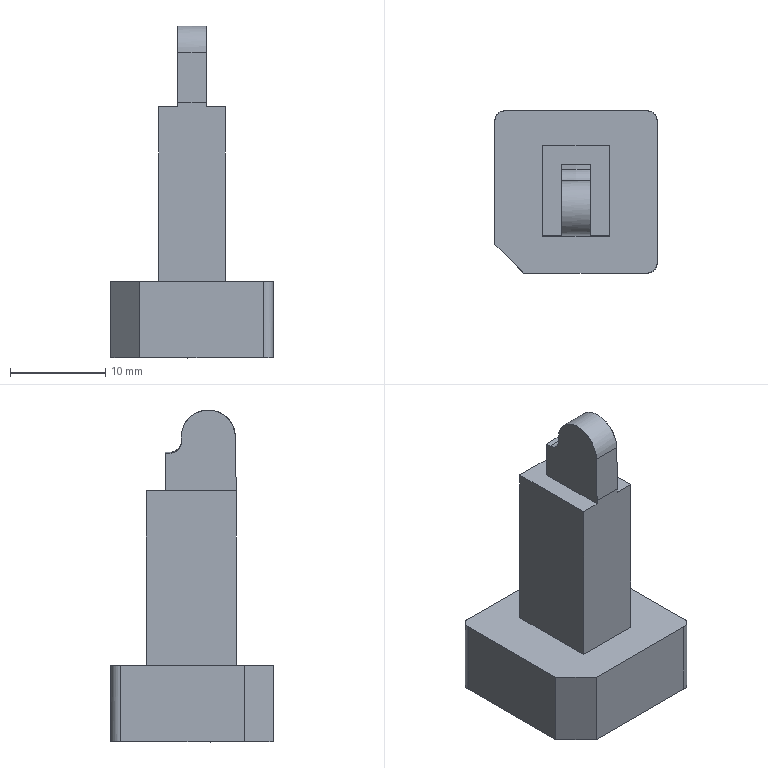NC program | PowerMill | posted with a generic post | part box 17 x 17 x 34.811 mm
Lines 7330 to 8096 of 55221:
N7427 M6
N7428 S18000 M03
N7429 G00 G90 X0.0 Y0.0
N7430 G43 Z10.798 H4
N7431
N7432 G05 P10000 R8
N7433 X1.6169 Y-5.4476
N7434 Z-2.5513
N7435 G01 Z-3.7513 F1200.0
N7436 X1.6122 Y-5.4523 Z-3.8139 F2000.0
N7437 X1.5599 Y-5.4621 Z-3.954
N7438 X1.5624 Y-5.4596 Z-3.8705
N7439 X1.5675 Y-5.4546 Z-3.7817
N7440 X1.5753 Y-5.4467 Z-3.6886
N7441 X1.5862 Y-5.4359 Z-3.5929
N7442 X1.5996 Y-5.4224 Z-3.4988
N7443 X1.6151 Y-5.4069 Z-3.4089
N7444 X1.6325 Y-5.3895 Z-3.3241
N7445 X1.6513 Y-5.3707 Z-3.245
N7446 X1.6713 Y-5.3507 Z-3.1717
N7447 X1.6895 Y-5.3325 Z-3.1127
N7448 X1.6972 Y-5.2824 Z-2.938
N7449 X1.6768 Y-5.3028 Z-2.9919
N7450 X1.6562 Y-5.3234 Z-3.0525
N7451 X1.6353 Y-5.3443 Z-3.121
N7452 X1.613 Y-5.3666 Z-3.2028
N7453 X1.5942 Y-5.3854 Z-3.2805
N7454 X1.5799 Y-5.3997 Z-3.3468
N7455 X1.5677 Y-5.4119 Z-3.4119
N7456 X1.5571 Y-5.4225 Z-3.4775
N7457 X1.5452 Y-5.4343 Z-3.5594
N7458 X1.5353 Y-5.4443 Z-3.6419
N7459 X1.5274 Y-5.4522 Z-3.7248
N7460 X1.5213 Y-5.4583 Z-3.8138
N7461 X1.5176 Y-5.462 Z-3.8974
N7462 X1.5152 Y-5.4644 Z-3.9811
N7463 X1.5138 Y-5.4658 Z-4.0648
N7464 X1.4711 Y-5.4661 Z-4.0801
N7465 X1.4724 Y-5.4647 Z-3.9923
N7466 X1.4748 Y-5.4623 Z-3.9046
N7467 X1.4789 Y-5.4582 Z-3.8131
N7468 X1.4857 Y-5.4515 Z-3.7139
N7469 X1.4939 Y-5.4433 Z-3.627
N7470 X1.5043 Y-5.4328 Z-3.5406
N7471 X1.5169 Y-5.4203 Z-3.4547
N7472 X1.5303 Y-5.4068 Z-3.375
N7473 X1.5485 Y-5.3887 Z-3.2817
N7474 X1.5684 Y-5.3688 Z-3.1934
N7475 X1.5901 Y-5.3471 Z-3.1096
N7476 X1.6136 Y-5.3236 Z-3.0299
N7477 X1.6389 Y-5.2982 Z-2.9538
N7478 X1.6662 Y-5.271 Z-2.8811
N7479 X1.6957 Y-5.2415 Z-2.8107
N7480 X1.6994 Y-5.2377 Z-2.8022
N7481 X1.7034 Y-5.1913 Z-2.6787
N7482 X1.7001 Y-5.1946 Z-2.6853
N7483 X1.6691 Y-5.2256 Z-2.7504
N7484 X1.6397 Y-5.255 Z-2.819
N7485 X1.612 Y-5.2827 Z-2.8914
N7486 X1.5859 Y-5.3088 Z-2.9678
N7487 X1.5615 Y-5.3332 Z-3.0484
N7488 X1.5388 Y-5.356 Z-3.1333
N7489 X1.5178 Y-5.377 Z-3.2229
N7490 X1.5022 Y-5.3926 Z-3.2983
N7491 X1.4862 Y-5.4085 Z-3.3835
N7492 X1.472 Y-5.4227 Z-3.4694
N7493 X1.4598 Y-5.4349 Z-3.5558
N7494 X1.4498 Y-5.445 Z-3.6429
N7495 X1.4413 Y-5.4535 Z-3.7396
N7496 X1.4356 Y-5.4592 Z-3.8308
N7497 X1.4319 Y-5.4629 Z-3.9189
N7498 X1.4296 Y-5.4652 Z-4.0072
N7499 X1.4284 Y-5.4664 Z-4.0954
N7500 X1.3857 Y-5.4666 Z-4.1108
N7501 X1.3871 Y-5.4653 Z-4.0237
N7502 X1.3891 Y-5.4632 Z-3.9366
N7503 X1.3925 Y-5.4598 Z-3.8464
N7504 X1.3975 Y-5.4548 Z-3.7596
N7505 X1.4046 Y-5.4477 Z-3.6732
N7506 X1.4137 Y-5.4386 Z-3.5871
N7507 X1.4247 Y-5.4276 Z-3.5015
N7508 X1.4381 Y-5.4143 Z-3.4146
N7509 X1.4535 Y-5.3988 Z-3.3285
N7510 X1.473 Y-5.3793 Z-3.2328
N7511 X1.4932 Y-5.3591 Z-3.1441
N7512 X1.5142 Y-5.3381 Z-3.0603
N7513 X1.53 Y-5.3223 Z-3.0031
N7514 X1.5467 Y-5.3056 Z-2.9476
N7515 X1.5651 Y-5.2872 Z-2.892
N7516 X1.5886 Y-5.2637 Z-2.8266
N7517 X1.6187 Y-5.2336 Z-2.7504
N7518 X1.646 Y-5.2063 Z-2.6873
N7519 X1.6707 Y-5.1816 Z-2.6353
N7520 X1.696 Y-5.1563 Z-2.5869
N7521 X1.706 Y-5.1463 Z-2.5692
N7522 X1.7074 Y-5.1025 Z-2.4708
N7523 X1.6942 Y-5.1157 Z-2.4924
N7524 X1.6649 Y-5.145 Z-2.5445
N7525 X1.6352 Y-5.1747 Z-2.6031
N7526 X1.6052 Y-5.2047 Z-2.6685
N7527 X1.5751 Y-5.2348 Z-2.7412
N7528 X1.5453 Y-5.2646 Z-2.8208
N7529 X1.5167 Y-5.2932 Z-2.9054
N7530 X1.4917 Y-5.3182 Z-2.9872
N7531 X1.4707 Y-5.3392 Z-3.0631
N7532 X1.453 Y-5.3569 Z-3.1332
N7533 X1.4332 Y-5.3767 Z-3.2199
N7534 X1.4137 Y-5.3962 Z-3.3152
N7535 X1.3962 Y-5.4137 Z-3.4123
N7536 X1.3825 Y-5.4274 Z-3.5013
N7537 X1.3726 Y-5.4373 Z-3.5779
N7538 X1.3641 Y-5.4458 Z-3.6548
N7539 X1.3571 Y-5.4528 Z-3.7319
N7540 X1.3518 Y-5.4581 Z-3.8093
N7541 X1.348 Y-5.4619 Z-3.8925
N7542 X1.3458 Y-5.4641 Z-3.9704
N7543 X1.3443 Y-5.4656 Z-4.0483
N7544 X1.343 Y-5.4669 Z-4.1261
N7545 X1.3005 Y-5.467 Z-4.1313
N7546 X1.3019 Y-5.4655 Z-4.0456
N7547 X1.3037 Y-5.4638 Z-3.9598
N7548 X1.3072 Y-5.4603 Z-3.8565
N7549 X1.3118 Y-5.4557 Z-3.7711
N7550 X1.3184 Y-5.4491 Z-3.6861
N7551 X1.3271 Y-5.4404 Z-3.6013
N7552 X1.3377 Y-5.4297 Z-3.517
N7553 X1.3533 Y-5.4141 Z-3.4142
N7554 X1.3717 Y-5.3958 Z-3.3125
N7555 X1.3927 Y-5.3747 Z-3.2119
N7556 X1.4164 Y-5.351 Z-3.1124
N7557 X1.4433 Y-5.3241 Z-3.0106
N7558 X1.4715 Y-5.296 Z-2.9141
N7559 X1.5006 Y-5.2669 Z-2.824
N7560 X1.5305 Y-5.237 Z-2.7403
N7561 X1.5611 Y-5.2064 Z-2.6627
N7562 X1.5924 Y-5.1751 Z-2.5909
N7563 X1.6244 Y-5.1431 Z-2.5246
N7564 X1.6571 Y-5.1103 Z-2.4633
N7565 X1.6906 Y-5.0769 Z-2.407
N7566 X1.7078 Y-5.0597 Z-2.3802
N7567 X1.7082 Y-5.0168 Z-2.2964
N7568 X1.6964 Y-5.0287 Z-2.3131
N7569 X1.6667 Y-5.0584 Z-2.3584
N7570 X1.6359 Y-5.0891 Z-2.4103
N7571 X1.6032 Y-5.1218 Z-2.4712
N7572 X1.5698 Y-5.1552 Z-2.5395
N7573 X1.5418 Y-5.1832 Z-2.6022
N7574 X1.519 Y-5.206 Z-2.6578
N7575 X1.4911 Y-5.234 Z-2.731
N7576 X1.4589 Y-5.2661 Z-2.8224
N7577 X1.4276 Y-5.2974 Z-2.9196
N7578 X1.3979 Y-5.3271 Z-3.0212
N7579 X1.3709 Y-5.3541 Z-3.124
N7580 X1.3472 Y-5.3778 Z-3.2252
N7581 X1.327 Y-5.398 Z-3.3231
N7582 X1.3101 Y-5.415 Z-3.4179
N7583 X1.297 Y-5.428 Z-3.504
N7584 X1.286 Y-5.4391 Z-3.5905
N7585 X1.2769 Y-5.4481 Z-3.6775
N7586 X1.27 Y-5.4551 Z-3.7648
N7587 X1.265 Y-5.46 Z-3.8526
N7588 X1.2613 Y-5.4637 Z-3.9551
N7589 X1.2594 Y-5.4657 Z-4.0432
N7590 X1.2581 Y-5.467 Z-4.1313
N7591 X1.2156
N7592 X1.2169 Y-5.4657 Z-4.0474
N7593 X1.2187 Y-5.4639 Z-3.9635
N7594 X1.2214 Y-5.4612 Z-3.8775
N7595 X1.226 Y-5.4566 Z-3.786
N7596 X1.2322 Y-5.4504 Z-3.7027
N7597 X1.2403 Y-5.4423 Z-3.6197
N7598 X1.2503 Y-5.4323 Z-3.5371
N7599 X1.2621 Y-5.4206 Z-3.4549
N7600 X1.2774 Y-5.4053 Z-3.3629
N7601 X1.2966 Y-5.386 Z-3.2626
N7602 X1.3181 Y-5.3645 Z-3.1645
N7603 X1.34 Y-5.3426 Z-3.076
N7604 X1.3643 Y-5.3183 Z-2.9887
N7605 X1.3976 Y-5.285 Z-2.8803
N7606 X1.4326 Y-5.25 Z-2.776
N7607 X1.4692 Y-5.2134 Z-2.6757
N7608 X1.5026 Y-5.18 Z-2.5919
N7609 X1.5363 Y-5.1463 Z-2.5148
N7610 X1.5704 Y-5.1122 Z-2.4437
N7611 X1.6051 Y-5.0775 Z-2.3779
N7612 X1.6406 Y-5.0421 Z-2.3172
N7613 X1.6768 Y-5.0059 Z-2.261
N7614 X1.7085 Y-4.9741 Z-2.2162
N7615 X1.7087 Y-4.9314 Z-2.1427
N7616 X1.7079 Y-4.9322 Z-2.1437
N7617 X1.6773 Y-4.9629 Z-2.1831
N7618 X1.6464 Y-4.9937 Z-2.2273
N7619 X1.613 Y-5.0272 Z-2.2804
N7620 X1.5775 Y-5.0626 Z-2.3422
N7621 X1.5477 Y-5.0925 Z-2.3991
N7622 X1.5234 Y-5.1168 Z-2.449
N7623 X1.4946 Y-5.1456 Z-2.512
N7624 X1.4546 Y-5.1856 Z-2.6059
N7625 X1.4169 Y-5.2233 Z-2.702
N7626 X1.3817 Y-5.2585 Z-2.8001
N7627 X1.3489 Y-5.2913 Z-2.9003
N7628 X1.3186 Y-5.3216 Z-3.0023
N7629 X1.2944 Y-5.3458 Z-3.0914
N7630 X1.2721 Y-5.3681 Z-3.1816
N7631 X1.2515 Y-5.3887 Z-3.2751
N7632 X1.2329 Y-5.4073 Z-3.372
N7633 X1.2175 Y-5.4226 Z-3.4665
N7634 X1.2049 Y-5.4353 Z-3.5603
N7635 X1.1946 Y-5.4456 Z-3.6547
N7636 X1.1876 Y-5.4526 Z-3.7337
N7637 X1.1821 Y-5.4581 Z-3.8129
N7638 X1.1782 Y-5.462 Z-3.8923
N7639 X1.1759 Y-5.4643 Z-3.9719
N7640 X1.1744 Y-5.4658 Z-4.0516
N7641 X1.1732 Y-5.467 Z-4.1313
N7642 X1.1308
N7643 X1.1321 Y-5.4657 Z-4.0474
N7644 X1.1338 Y-5.4639 Z-3.9634
N7645 X1.1365 Y-5.4613 Z-3.8796
N7646 X1.1411 Y-5.4567 Z-3.7879
N7647 X1.1472 Y-5.4506 Z-3.7046
N7648 X1.1553 Y-5.4425 Z-3.6216
N7649 X1.1652 Y-5.4326 Z-3.5389
N7650 X1.1768 Y-5.421 Z-3.4567
N7651 X1.1926 Y-5.4052 Z-3.3618
N7652 X1.2118 Y-5.3859 Z-3.2624
N7653 X1.2337 Y-5.364 Z-3.1638
N7654 X1.2568 Y-5.341 Z-3.0719
N7655 X1.2796 Y-5.3182 Z-2.9905
N7656 X1.3035 Y-5.2943 Z-2.9098
N7657 X1.3287 Y-5.269 Z-2.8298
N7658 X1.3561 Y-5.2416 Z-2.7513
N7659 X1.3855 Y-5.2122 Z-2.6743
N7660 X1.4134 Y-5.1844 Z-2.6047
N7661 X1.4536 Y-5.1441 Z-2.5088
N7662 X1.4915 Y-5.1063 Z-2.4252
N7663 X1.5281 Y-5.0696 Z-2.3507
N7664 X1.5643 Y-5.0335 Z-2.2834
N7665 X1.6003 Y-4.9974 Z-2.2223
N7666 X1.6366 Y-4.9611 Z-2.1666
N7667 X1.6733 Y-4.9244 Z-2.1158
N7668 X1.7082 Y-4.8895 Z-2.0723
N7669 X1.7081 Y-4.8472 Z-2.005
N7670 X1.6852 Y-4.8701 Z-2.0313
N7671 X1.6499 Y-4.9054 Z-2.0761
N7672 X1.6138 Y-4.9415 Z-2.1269
N7673 X1.5768 Y-4.9785 Z-2.1845
N7674 X1.5388 Y-5.0165 Z-2.2493
N7675 X1.4998 Y-5.0556 Z-2.3218
N7676 X1.4607 Y-5.0946 Z-2.4001
N7677 X1.4296 Y-5.1257 Z-2.4669
N7678 X1.3953 Y-5.16 Z-2.5456
N7679 X1.3624 Y-5.1929 Z-2.6255
N7680 X1.3238 Y-5.2315 Z-2.7257
N7681 X1.2941 Y-5.2612 Z-2.8083
N7682 X1.2662 Y-5.2891 Z-2.8918
N7683 X1.2408 Y-5.3145 Z-2.975
N7684 X1.2176 Y-5.3377 Z-3.0594
N7685 X1.1962 Y-5.3591 Z-3.1448
N7686 X1.1729 Y-5.3824 Z-3.2474
N7687 X1.1553 Y-5.4 Z-3.3345
N7688 X1.1397 Y-5.4156 Z-3.4224
N7689 X1.1269 Y-5.4284 Z-3.5076
N7690 X1.1159 Y-5.4394 Z-3.5933
N7691 X1.107 Y-5.4483 Z-3.6794
N7692 X1.1002 Y-5.4551 Z-3.7659
N7693 X1.0947 Y-5.4607 Z-3.8666
N7694 X1.0915 Y-5.4638 Z-3.9569
N7695 X1.0896 Y-5.4657 Z-4.0441
N7696 X1.0883 Y-5.467 Z-4.1313
N7697 X1.0459
N7698 X1.0472 Y-5.4657 Z-4.0475
N7699 X1.0489 Y-5.464 Z-3.9637
N7700 X1.0516 Y-5.4613 Z-3.8799
N7701 X1.0557 Y-5.4572 Z-3.7964
N7702 X1.0616 Y-5.4513 Z-3.7131
N7703 X1.0695 Y-5.4434 Z-3.6301
N7704 X1.0792 Y-5.4337 Z-3.5475
N7705 X1.0934 Y-5.4195 Z-3.4478
N7706 X1.1107 Y-5.4022 Z-3.3468
N7707 X1.131 Y-5.3819 Z-3.2447
N7708 X1.1545 Y-5.3584 Z-3.1412
N7709 X1.1782 Y-5.3347 Z-3.0479
N7710 X1.2042 Y-5.3087 Z-2.9559
N7711 X1.2331 Y-5.2798 Z-2.8634
N7712 X1.2661 Y-5.2468 Z-2.767
N7713 X1.3033 Y-5.2096 Z-2.6675
N7714 X1.344 Y-5.1689 Z-2.5668
N7715 X1.3866 Y-5.1263 Z-2.4692
N7716 X1.4294 Y-5.0834 Z-2.3778
N7717 X1.4717 Y-5.0412 Z-2.2937
N7718 X1.4955 Y-5.0174 Z-2.2488
N7719 X1.5235 Y-4.9894 Z-2.1988
N7720 X1.5582 Y-4.9547 Z-2.1408
N7721 X1.5977 Y-4.9152 Z-2.0798
N7722 X1.6334 Y-4.8795 Z-2.0294
N7723 X1.6655 Y-4.8474 Z-1.988
N7724 X1.696 Y-4.8169 Z-1.9525
N7725 X1.7089 Y-4.804 Z-1.9388
N7726 X1.7087 Y-4.7618 Z-1.8785
N7727 X1.6856 Y-4.7848 Z-1.9024
N7728 X1.6489 Y-4.8216 Z-1.9443
N7729 X1.6119 Y-4.8586 Z-1.9915
N7730 X1.5745 Y-4.8959 Z-2.0442
N7731 X1.5365 Y-4.9339 Z-2.103
N7732 X1.4978 Y-4.9727 Z-2.1682
N7733 X1.4588 Y-5.0117 Z-2.2385
N7734 X1.411 Y-5.0595 Z-2.33
N7735 X1.3638 Y-5.1067 Z-2.4269
N7736 X1.3195 Y-5.151 Z-2.5248
N7737 X1.2783 Y-5.1922 Z-2.6228
N7738 X1.2405 Y-5.23 Z-2.7204
N7739 X1.2061 Y-5.2643 Z-2.817
N7740 X1.1753 Y-5.2952 Z-2.9123
N7741 X1.1469 Y-5.3236 Z-3.0083
N7742 X1.1205 Y-5.35 Z-3.1064
N7743 X1.0983 Y-5.3721 Z-3.1988
N7744 X1.0812 Y-5.3893 Z-3.2801
N7745 X1.0657 Y-5.4048 Z-3.3621
N7746 X1.0516 Y-5.4188 Z-3.4446
N7747 X1.0393 Y-5.4312 Z-3.5275
N7748 X1.0289 Y-5.4415 Z-3.611
N7749 X1.0203 Y-5.4501 Z-3.6986
N7750 X1.0136 Y-5.4569 Z-3.7917
N7751 X1.0094 Y-5.4611 Z-3.8765
N7752 X1.0065 Y-5.464 Z-3.9614
N7753 X1.0047 Y-5.4658 Z-4.0464
N7754 X1.0035 Y-5.467 Z-4.1313
N7755 X0.9611
N7756 X0.9624 Y-5.4657 Z-4.0517
N7757 X0.964 Y-5.464 Z-3.9722
N7758 X0.9663 Y-5.4617 Z-3.8926
N7759 X0.9698 Y-5.4583 Z-3.8132
N7760 X0.9755 Y-5.4526 Z-3.7266
N7761 X0.9827 Y-5.4454 Z-3.6478
N7762 X0.9917 Y-5.4363 Z-3.5694
N7763 X1.0023 Y-5.4257 Z-3.4914
N7764 X1.0142 Y-5.4138 Z-3.4138
N7765 X1.0275 Y-5.4005 Z-3.3365
N7766 X1.0464 Y-5.3817 Z-3.2423
N7767 X1.0689 Y-5.3592 Z-3.1441
N7768 X1.0949 Y-5.3331 Z-3.0428
N7769 X1.1235 Y-5.3045 Z-2.9427
N7770 X1.155 Y-5.273 Z-2.8431
N7771 X1.1894 Y-5.2386 Z-2.744
N7772 X1.2268 Y-5.2013 Z-2.6455
N7773 X1.267 Y-5.161 Z-2.5477
N7774 X1.3102 Y-5.1179 Z-2.4507
N7775 X1.3563 Y-5.0718 Z-2.3546
N7776 X1.4053 Y-5.0227 Z-2.2595
N7777 X1.4426 Y-4.9855 Z-2.1914
N7778 X1.4806 Y-4.9474 Z-2.1246
N7779 X1.5218 Y-4.9063 Z-2.0565
N7780 X1.5606 Y-4.8674 Z-1.9973
N7781 X1.5977 Y-4.8304 Z-1.9458
N7782 X1.6336 Y-4.7944 Z-1.9004
N7783 X1.6711 Y-4.7569 Z-1.8576
N7784 X1.7087 Y-4.7193 Z-1.8185
N7785 X1.7096 Y-4.6761 Z-1.7608
N7786 X1.6713 Y-4.7143 Z-1.7985
N7787 X1.6312 Y-4.7544 Z-1.8426
N7788 X1.5918 Y-4.7938 Z-1.8911
N7789 X1.553 Y-4.8327 Z-1.944
N7790 X1.5048 Y-4.8808 Z-2.0157
N7791 X1.456 Y-4.9297 Z-2.0941
N7792 X1.4059 Y-4.9797 Z-2.1802
N7793 X1.3679 Y-5.0177 Z-2.2494
N7794 X1.3308 Y-5.0548 Z-2.3196
N7795 X1.295 Y-5.0906 Z-2.3911
N7796 X1.2611 Y-5.1246 Z-2.4644
N7797 X1.2286 Y-5.157 Z-2.5391
N7798 X1.197 Y-5.1886 Z-2.6145
N7799 X1.1626 Y-5.223 Z-2.7016
N7800 X1.1304 Y-5.2552 Z-2.7904
N7801 X1.0974 Y-5.2882 Z-2.8894
N7802 X1.0691 Y-5.3165 Z-2.9824
N7803 X1.0435 Y-5.3421 Z-3.0754
N7804 X1.0202 Y-5.3654 Z-3.1697
N7805 X0.9982 Y-5.3874 Z-3.2707
N7806 X0.9786 Y-5.4071 Z-3.3741
N7807 X0.9617 Y-5.4239 Z-3.4781
N7808 X0.9478 Y-5.4378 Z-3.5816
N7809 X0.9369 Y-5.4487 Z-3.6838
N7810 X0.9289 Y-5.4568 Z-3.7844
N7811 X0.9246 Y-5.461 Z-3.8664
N7812 X0.9221 Y-5.4635 Z-3.9486
N7813 X0.9201 Y-5.4655 Z-4.049
N7814 X0.9186 Y-5.467 Z-4.1313
N7815 X0.8762
N7816 X0.8778 Y-5.4654 Z-4.0385
N7817 X0.8796 Y-5.4636 Z-3.9458
N7818 X0.8827 Y-5.4605 Z-3.8532
N7819 X0.888 Y-5.4552 Z-3.7608
N7820 X0.8962 Y-5.447 Z-3.6633
N7821 X0.9075 Y-5.4356 Z-3.563
N7822 X0.922 Y-5.4212 Z-3.4595
N7823 X0.9389 Y-5.4043 Z-3.358
N7824 X0.9587 Y-5.3845 Z-3.2566
N7825 X0.9813 Y-5.3619 Z-3.1551
N7826 X1.007 Y-5.3362 Z-3.0534
N7827 X1.0346 Y-5.3086 Z-2.9551
N7828 X1.0651 Y-5.2781 Z-2.8575
N7829 X1.0987 Y-5.2445 Z-2.7597
N7830 X1.1354 Y-5.2078 Z-2.6618
N7831 X1.1753 Y-5.1679 Z-2.5641
N7832 X1.2182 Y-5.125 Z-2.4664
N7833 X1.2626 Y-5.0806 Z-2.3719
N7834 X1.3059 Y-5.0373 Z-2.2863
N7835 X1.3494 Y-4.9938 Z-2.2061
N7836 X1.4046 Y-4.9386 Z-2.1094
N7837 X1.4544 Y-4.8888 Z-2.0273
N7838 X1.5013 Y-4.8419 Z-1.9553
N7839 X1.5464 Y-4.7968 Z-1.8912
N7840 X1.5904 Y-4.7528 Z-1.8338
N7841 X1.63 Y-4.7132 Z-1.7863
N7842 X1.6647 Y-4.6785 Z-1.7486
N7843 X1.6969 Y-4.6463 Z-1.7178
N7844 X1.7092 Y-4.634 Z-1.7073
N7845 X1.7087 Y-4.5921 Z-1.6545
N7846 X1.6904 Y-4.6104 Z-1.6708
N7847 X1.6524 Y-4.6484 Z-1.7072
N7848 X1.6142 Y-4.6865 Z-1.7475
N7849 X1.5749 Y-4.7258 Z-1.7934
N7850 X1.5342 Y-4.7666 Z-1.8459
N7851 X1.495 Y-4.8057 Z-1.901
N7852 X1.4589 Y-4.8418 Z-1.9552
N7853 X1.4251 Y-4.8757 Z-2.0083
N7854 X1.3926 Y-4.9082 Z-2.0607
N7855 X1.36 Y-4.9408 Z-2.1143
N7856 X1.3087 Y-4.9921 Z-2.2033
N7857 X1.2586 Y-5.0421 Z-2.2962
N7858 X1.2106 Y-5.0902 Z-2.3921
N7859 X1.1653 Y-5.1355 Z-2.4893
N7860 X1.1231 Y-5.1777 Z-2.5869
N7861 X1.0839 Y-5.2169 Z-2.685
N7862 X1.0507 Y-5.2501 Z-2.7755
N7863 X1.0183 Y-5.2825 Z-2.8724
N7864 X0.9863 Y-5.3145 Z-2.9772
N7865 X0.9608 Y-5.3399 Z-3.0682
N7866 X0.9375 Y-5.3633 Z-3.1612
N7867 X0.9151 Y-5.3857 Z-3.2618
N7868 X0.8958 Y-5.405 Z-3.361
N7869 X0.8799 Y-5.4209 Z-3.4563
N7870 X0.8682 Y-5.4325 Z-3.5386
N7871 X0.8583 Y-5.4424 Z-3.6213
N7872 X0.8502 Y-5.4505 Z-3.7043
N7873 X0.8441 Y-5.4567 Z-3.7877
N7874 X0.8395 Y-5.4613 Z-3.8794
N7875 X0.8368 Y-5.4639 Z-3.9633
N7876 X0.8351 Y-5.4657 Z-4.0473
N7877 X0.8338 Y-5.467 Z-4.1313
N7878 X0.7914
N7879 X0.7926 Y-5.4657 Z-4.0455
N7880 X0.7945 Y-5.4639 Z-3.9598
N7881 X0.7977 Y-5.4607 Z-3.8653
N7882 X0.8027 Y-5.4557 Z-3.7722
N7883 X0.8093 Y-5.449 Z-3.6871
N7884 X0.818 Y-5.4404 Z-3.6024
N7885 X0.8286 Y-5.4297 Z-3.5182
N7886 X0.8411 Y-5.4173 Z-3.4343
N7887 X0.859 Y-5.3993 Z-3.3311
N7888 X0.8797 Y-5.3786 Z-3.2289
N7889 X0.9031 Y-5.3552 Z-3.1277
N7890 X0.9292 Y-5.3291 Z-3.0276
N7891 X0.958 Y-5.3003 Z-2.9288
N7892 X0.9894 Y-5.2689 Z-2.8313
N7893 X1.0243 Y-5.2341 Z-2.7321
N7894 X1.0617 Y-5.1967 Z-2.6342
N7895 X1.1017 Y-5.1566 Z-2.5373
N7896 X1.1446 Y-5.1138 Z-2.4416
N7897 X1.1903 Y-5.0681 Z-2.3468
N7898 X1.2389 Y-5.0194 Z-2.253
N7899 X1.2906 Y-4.9678 Z-2.16
N7900 X1.3453 Y-4.9131 Z-2.0679
N7901 X1.4029 Y-4.8554 Z-1.9765
N7902 X1.4592 Y-4.7992 Z-1.8918
N7903 X1.5053 Y-4.753 Z-1.8262
N7904 X1.547 Y-4.7113 Z-1.7714
N7905 X1.5866 Y-4.6717 Z-1.7239
N7906 X1.626 Y-4.6323 Z-1.681
N7907 X1.6669 Y-4.5915 Z-1.6409
N7908 X1.7069 Y-4.5515 Z-1.6058
N7909 X1.7048 Y-4.5111 Z-1.5579
N7910 X1.6629 Y-4.553 Z-1.5939
N7911 X1.6193 Y-4.5966 Z-1.6356
N7912 X1.579 Y-4.6369 Z-1.6787
N7913 X1.5418 Y-4.6742 Z-1.7232
N7914 X1.4796 Y-4.7363 Z-1.8043
N7915 X1.4187 Y-4.7972 Z-1.8891
N7916 X1.3594 Y-4.8565 Z-1.9773
N7917 X1.302 Y-4.9139 Z-2.0684
N7918 X1.2471 Y-4.9689 Z-2.1617
N7919 X1.1947 Y-5.0212 Z-2.2567
N7920 X1.1452 Y-5.0707 Z-2.353
N7921 X1.1007 Y-5.1153 Z-2.4456
N7922 X1.0583 Y-5.1576 Z-2.5397
N7923 X1.0185 Y-5.1975 Z-2.6355
N7924 X0.9815 Y-5.2344 Z-2.7319
N7925 X0.9475 Y-5.2684 Z-2.8287
N7926 X0.9165 Y-5.2994 Z-2.9258
N7927 X0.8883 Y-5.3276 Z-3.0231
N7928 X0.8625 Y-5.3534 Z-3.1213
N7929 X0.8392 Y-5.3767 Z-3.2207
N7930 X0.8184 Y-5.3975 Z-3.321
N7931 X0.8008 Y-5.4151 Z-3.4194
N7932 X0.7879 Y-5.4281 Z-3.5048
N7933 X0.7768 Y-5.4391 Z-3.5906
N7934 X0.7678 Y-5.4481 Z-3.6769
N7935 X0.7609 Y-5.455 Z-3.7636
N7936 X0.7557 Y-5.4602 Z-3.8561
N7937 X0.7522 Y-5.4638 Z-3.9565
N7938 X0.7503 Y-5.4657 Z-4.0439
N7939 X0.7489 Y-5.467 Z-4.1313
N7940 X0.7065
N7941 X0.7077 Y-5.4658 Z-4.0554
N7942 X0.7091 Y-5.4644 Z-3.9794
N7943 X0.7111 Y-5.4624 Z-3.9035
N7944 X0.7142 Y-5.4592 Z-3.8277
N7945 X0.719 Y-5.4545 Z-3.7522
N7946 X0.7255 Y-5.448 Z-3.6769
N7947 X0.7336 Y-5.4399 Z-3.602
N7948 X0.743 Y-5.4305 Z-3.5273
N7949 X0.7535 Y-5.42 Z-3.4529
N7950 X0.769 Y-5.4045 Z-3.3588
N7951 X0.7871 Y-5.3863 Z-3.2645
N7952 X0.8075 Y-5.366 Z-3.1724
N7953 X0.83 Y-5.3435 Z-3.0811
N7954 X0.8558 Y-5.3177 Z-2.987
N7955 X0.8844 Y-5.2891 Z-2.8926
N7956 X0.9169 Y-5.2566 Z-2.795
N7957 X0.9533 Y-5.2202 Z-2.6952
N7958 X0.993 Y-5.1805 Z-2.5947
N7959 X1.035 Y-5.1385 Z-2.4964
N7960 X1.0779 Y-5.0956 Z-2.4031
N7961 X1.1208 Y-5.0526 Z-2.3161
N7962 X1.1644 Y-5.009 Z-2.2336
N7963 X1.218 Y-4.9555 Z-2.1385
N7964 X1.2741 Y-4.8994 Z-2.0452
N7965 X1.3327 Y-4.8408 Z-1.954
N7966 X1.3937 Y-4.7798 Z-1.865
N7967 X1.4466 Y-4.7269 Z-1.7914
N7968 X1.497 Y-4.6765 Z-1.7244
N7969 X1.5419 Y-4.6316 Z-1.6688
N7970 X1.5836 Y-4.5899 Z-1.6218
N7971 X1.6235 Y-4.55 Z-1.581
N7972 X1.664 Y-4.5095 Z-1.544
N7973 X1.7045 Y-4.469 Z-1.5111
N7974 Y-4.4266 Z-1.466
N7975 X1.6834 Y-4.4477 Z-1.4811
N7976 X1.6531 Y-4.478 Z-1.5057
N7977 X1.6218 Y-4.5093 Z-1.5341
N7978 X1.5875 Y-4.5435 Z-1.5683
N7979 X1.5497 Y-4.5814 Z-1.6092
N7980 X1.5072 Y-4.6238 Z-1.6584
N7981 X1.4585 Y-4.6725 Z-1.7188
N7982 X1.4015 Y-4.7296 Z-1.7942
N7983 X1.3527 Y-4.7783 Z-1.8622
N7984 X1.3133 Y-4.8178 Z-1.9197
N7985 X1.2803 Y-4.8508 Z-1.9694
N7986 X1.2522 Y-4.8788 Z-2.0129
N7987 X1.1981 Y-4.9329 Z-2.1005
N7988 X1.1442 Y-4.9869 Z-2.1937
N7989 X1.0933 Y-5.0378 Z-2.2877
N7990 X1.0453 Y-5.0857 Z-2.3828
N7991 X1.0003 Y-5.1308 Z-2.4788
N7992 X0.9581 Y-5.173 Z-2.5759
N7993 X0.9187 Y-5.2123 Z-2.674
N7994 X0.8821 Y-5.249 Z-2.7732
N7995 X0.8481 Y-5.283 Z-2.8738
N7996 X0.8166 Y-5.3144 Z-2.9761
N7997 X0.7907 Y-5.3403 Z-3.0691
N7998 X0.767 Y-5.364 Z-3.1642
N7999 X0.7447 Y-5.3864 Z-3.2655
N8000 X0.7253 Y-5.4058 Z-3.366
N8001 X0.7092 Y-5.4219 Z-3.4633
N8002 X0.6978 Y-5.4332 Z-3.5446
N8003 X0.6881 Y-5.443 Z-3.6262
N8004 X0.6802 Y-5.4509 Z-3.7083
N8005 X0.6742 Y-5.4569 Z-3.7906
N8006 X0.6696 Y-5.4614 Z-3.8826
N8007 X0.6671 Y-5.464 Z-3.9654
N8008 X0.6654 Y-5.4657 Z-4.0484
N8009 X0.6641 Y-5.467 Z-4.1313
N8010 X0.6217
N8011 X0.6227 Y-5.4659 Z-4.042
N8012 X0.6248 Y-5.4639 Z-3.9527
N8013 X0.6283 Y-5.4604 Z-3.8597
N8014 X0.6339 Y-5.4547 Z-3.7611
N8015 X0.6423 Y-5.4464 Z-3.6597
N8016 X0.6525 Y-5.4361 Z-3.5658
N8017 X0.6644 Y-5.4242 Z-3.4783
N8018 X0.6784 Y-5.4102 Z-3.3914
N8019 X0.6944 Y-5.3942 Z-3.3052
N8020 X0.7123 Y-5.3764 Z-3.2196
N8021 X0.7318 Y-5.3568 Z-3.1348
N8022 X0.7574 Y-5.3313 Z-3.0356
N8023 X0.786 Y-5.3027 Z-2.9363
N8024 X0.8175 Y-5.2711 Z-2.8372
N8025 X0.8521 Y-5.2365 Z-2.7382
N8026 X0.8897 Y-5.199 Z-2.6397
N8027 X0.9302 Y-5.1584 Z-2.5417
N8028 X0.9738 Y-5.1148 Z-2.4443
N8029 X1.0203 Y-5.0684 Z-2.3478
N8030 X1.0696 Y-5.019 Z-2.2524
N8031 X1.1218 Y-4.9668 Z-2.1583
N8032 X1.1766 Y-4.912 Z-2.0657
N8033 X1.235 Y-4.8536 Z-1.9731
N8034 X1.2941 Y-4.7945 Z-1.8851
N8035 X1.3539 Y-4.7347 Z-1.8017
N8036 X1.415 Y-4.6736 Z-1.7207
N8037 X1.471 Y-4.6176 Z-1.6495
N8038 X1.5193 Y-4.5693 Z-1.5921
N8039 X1.5636 Y-4.525 Z-1.5437
N8040 X1.6073 Y-4.4813 Z-1.5005
N8041 X1.6486 Y-4.4401 Z-1.4639
N8042 X1.688 Y-4.4006 Z-1.4331
N8043 X1.7047 Y-4.384 Z-1.4214
N8044 X1.7044 Y-4.3418 Z-1.3787
N8045 X1.6692 Y-4.3771 Z-1.4034
N8046 X1.6291 Y-4.4171 Z-1.4354
N8047 X1.5876 Y-4.4586 Z-1.473
N8048 X1.5442 Y-4.502 Z-1.5168
N8049 X1.4982 Y-4.548 Z-1.5675
N8050 X1.4501 Y-4.5961 Z-1.6245
N8051 X1.4065 Y-4.6397 Z-1.6782
N8052 X1.3534 Y-4.6928 Z-1.746
N8053 X1.2879 Y-4.7583 Z-1.8343
N8054 X1.2247 Y-4.8215 Z-1.9251
N8055 X1.1638 Y-4.8824 Z-2.0182
N8056 X1.1052 Y-4.941 Z-2.1137
N8057 X1.0626 Y-4.9836 Z-2.1871
N8058 X1.0217 Y-5.0245 Z-2.2624
N8059 X0.9823 Y-5.0639 Z-2.3393
N8060 X0.9382 Y-5.108 Z-2.4303
N8061 X0.8987 Y-5.1475 Z-2.517
N8062 X0.8639 Y-5.1823 Z-2.5982
N8063 X0.8309 Y-5.2153 Z-2.6809
N8064 X0.8 Y-5.2462 Z-2.7651
N8065 X0.7656 Y-5.2806 Z-2.8662
N8066 X0.7345 Y-5.3117 Z-2.9669
N8067 X0.7065 Y-5.3397 Z-3.0671
N8068 X0.6816 Y-5.3646 Z-3.1669
N8069 X0.6597 Y-5.3865 Z-3.2662
N8070 X0.6437 Y-5.4025 Z-3.3489
N8071 X0.6294 Y-5.4168 Z-3.4321
N8072 X0.6167 Y-5.4295 Z-3.5159
N8073 X0.606 Y-5.4402 Z-3.6001
N8074 X0.5974 Y-5.4489 Z-3.6849
N8075 X0.5902 Y-5.456 Z-3.7791
N8076 X0.5852 Y-5.461 Z-3.8739
N8077 X0.5823 Y-5.4639 Z-3.9597
N8078 X0.5804 Y-5.4658 Z-4.0455
N8079 X0.5792 Y-5.467 Z-4.1313
N8080 X0.5368
N8081 X0.5381 Y-5.4657 Z-4.047
N8082 X0.5399 Y-5.4639 Z-3.9627
N8083 X0.5426 Y-5.4612 Z-3.8785
N8084 X0.5472 Y-5.4566 Z-3.7869
N8085 X0.5533 Y-5.4504 Z-3.7032
N8086 X0.5615 Y-5.4423 Z-3.6199
N8087 X0.5715 Y-5.4323 Z-3.5369
N8088 X0.5832 Y-5.4206 Z-3.4544
N8089 X0.5991 Y-5.4047 Z-3.3595
N8090 X0.6184 Y-5.3854 Z-3.2606
N8091 X0.6408 Y-5.363 Z-3.1602
N8092 X0.6638 Y-5.34 Z-3.0683
N8093 X0.6891 Y-5.3146 Z-2.9777
N8094 X0.7212 Y-5.2825 Z-2.8727
N8095 X0.7538 Y-5.25 Z-2.7753
N8096 X0.7871 Y-5.2167 Z-2.6844
N8097 X0.8224 Y-5.1814 Z-2.596
N8098 X0.8648 Y-5.139 Z-2.4974
N8099 X0.9101 Y-5.0936 Z-2.3997
N8100 X0.9584 Y-5.0454 Z-2.3028
N8101 X1.0096 Y-4.9941 Z-2.207
N8102 X1.0638 Y-4.9399 Z-2.1121
N8103 X1.1166 Y-4.8871 Z-2.0253
N8104 X1.1733 Y-4.8305 Z-1.9379
N8105 X1.2342 Y-4.7696 Z-1.8498
N8106 X1.2978 Y-4.706 Z-1.7633
N8107 X1.36 Y-4.6438 Z-1.6837
N8108 X1.4212 Y-4.5825 Z-1.609
N8109 X1.4783 Y-4.5255 Z-1.5415
N8110 X1.5252 Y-4.4785 Z-1.4896
N8111 X1.5676 Y-4.4362 Z-1.4467
N8112 X1.6078 Y-4.396 Z-1.4099
N8113 X1.6482 Y-4.3556 Z-1.3768
N8114 X1.6897 Y-4.3141 Z-1.3466
N8115 X1.7046 Y-4.2991 Z-1.3367
N8116 X1.7076 Y-4.2538 Z-1.2945
N8117 X1.7074 Y-4.2539 Z-1.2946
N8118 X1.6652 Y-4.2961 Z-1.3226
N8119 X1.6215 Y-4.3399 Z-1.3559
N8120 X1.5763 Y-4.3851 Z-1.3947
N8121 X1.5307 Y-4.4307 Z-1.4383
N8122 X1.487 Y-4.4744 Z-1.4844
N8123 X1.4173 Y-4.544 Z-1.563
N8124 X1.3451 Y-4.6163 Z-1.6494
N8125 X1.2691 Y-4.6922 Z-1.7453
N8126 X1.2144 Y-4.747 Z-1.8179
N8127 X1.1587 Y-4.8027 Z-1.8969
N8128 X1.0994 Y-4.8619 Z-1.9863
N8129 X1.0414 Y-4.92 Z-2.0789
N8130 X0.9864 Y-4.9749 Z-2.1725
N8131 X0.9345 Y-5.0268 Z-2.2669
N8132 X0.8857 Y-5.0756 Z-2.3621
N8133 X0.84 Y-5.1214 Z-2.458
N8134 X0.7972 Y-5.1641 Z-2.5545
N8135 X0.7575 Y-5.2038 Z-2.6516
N8136 X0.7207 Y-5.2406 Z-2.7493
N8137 X0.687 Y-5.2743 Z-2.8469
N8138 X0.6555 Y-5.3058 Z-2.9469
N8139 X0.6272 Y-5.3342 Z-3.0464
N8140 X0.6019 Y-5.3595 Z-3.1456
N8141 X0.5793 Y-5.382 Z-3.2455
N8142 X0.5587 Y-5.4026 Z-3.3488
N8143 X0.5414 Y-5.42 Z-3.45
N8144 X0.5272 Y-5.4342 Z-3.5491
N8145 X0.5161 Y-5.4453 Z-3.6463
N8146 X0.5089 Y-5.4524 Z-3.7267
N8147 X0.5033 Y-5.458 Z-3.8073
N8148 X0.4994 Y-5.4619 Z-3.8881
N8149 X0.4971 Y-5.4643 Z-3.9691
N8150 X0.4956 Y-5.4657 Z-4.0502
N8151 X0.4944 Y-5.467 Z-4.1313
N8152 X0.4519
N8153 X0.4536 Y-5.4653 Z-4.0361
N8154 X0.4554 Y-5.4635 Z-3.9409
N8155 X0.4587 Y-5.4602 Z-3.8458
N8156 X0.4644 Y-5.4545 Z-3.751
N8157 X0.4731 Y-5.4458 Z-3.6523
N8158 X0.4848 Y-5.4342 Z-3.5515
N8159 X0.4995 Y-5.4194 Z-3.4483
N8160 X0.5173 Y-5.4017 Z-3.344
N8161 X0.5377 Y-5.3813 Z-3.2411
N8162 X0.5606 Y-5.3583 Z-3.1399
N8163 X0.5862 Y-5.3327 Z-3.0404
N8164 X0.6135 Y-5.3054 Z-2.9448
N8165 X0.6431 Y-5.2759 Z-2.8506
N8166 X0.6749 Y-5.2441 Z-2.7578
N8167 X0.7102 Y-5.2088 Z-2.6637
N8168 X0.7488 Y-5.1701 Z-2.5688
N8169 X0.7886 Y-5.1303 Z-2.4783
N8170 X0.8289 Y-5.09 Z-2.3923
N8171 X0.871 Y-5.0479 Z-2.3075
N8172 X0.9204 Y-4.9986 Z-2.2146
N8173 X0.9729 Y-4.946 Z-2.1222
N8174 X1.0287 Y-4.8902 Z-2.0305
N8175 X1.0878 Y-4.8311 Z-1.9394
N8176 X1.1444 Y-4.7745 Z-1.8572
N8177 X1.2057 Y-4.7132 Z-1.7727
N8178 X1.2693 Y-4.6497 Z-1.6901
N8179 X1.3341 Y-4.5849 Z-1.611
N8180 X1.3875 Y-4.5314 Z-1.5493
N8181 X1.434 Y-4.485 Z-1.497
N8182 X1.4892 Y-4.4297 Z-1.4367
N8183 X1.5347 Y-4.3842 Z-1.3905
N8184 X1.5754 Y-4.3435 Z-1.3529
N8185 X1.614 Y-4.3049 Z-1.3207
N8186 X1.6536 Y-4.2653 Z-1.2911
N8187 X1.6942 Y-4.2247 Z-1.2641
N8188 X1.7095 Y-4.2094 Z-1.2548
N8189 X1.7114 Y-4.1651 Z-1.2156
N8190 X1.7096 Y-4.1669 Z-1.2165
N8191 X1.6732 Y-4.2033 Z-1.2382
N8192 X1.6367 Y-4.2398 Z-1.2634
N8193 X1.5973 Y-4.2792 Z-1.2941